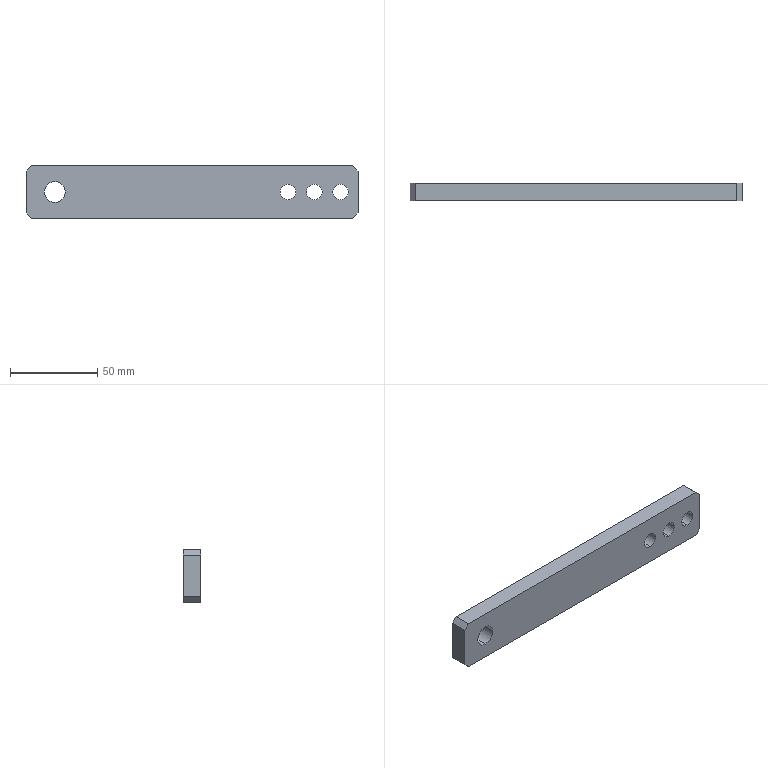Part | SolidWorks | features HoleWzd 2, Chamfer 1, Extrusion 1 | 1 solid | 18 faces | box 190 x 10 x 30 mm | volume 53781 mm3 | plane 10 | cylinder 8 | commonest cylinder face diameters 9 x6 12 x2
STEP:
#1=CARTESIAN_POINT('',(-78.492,10.,-6.));
#2=VERTEX_POINT('',#1);
#3=CARTESIAN_POINT('',(-78.492,10.,6.));
#4=VERTEX_POINT('',#3);
#5=CARTESIAN_POINT('',(-78.492,10.,0.));
#6=DIRECTION('',(0.,1.,0.));
#7=DIRECTION('',(0.,0.,1.));
#8=AXIS2_PLACEMENT_3D('',#5,#6,#7);
#9=CIRCLE('',#8,6.);
#10=EDGE_CURVE('',#2,#4,#9,.T.);
#11=ORIENTED_EDGE('',*,*,#10,.T.);
#12=CARTESIAN_POINT('',(-78.492,0.,6.));
#13=VERTEX_POINT('',#12);
#14=CARTESIAN_POINT('',(-78.492,0.,6.));
#15=DIRECTION('',(0.,-1.,0.));
#16=VECTOR('',#15,1000.);
#17=LINE('',#14,#16);
#18=EDGE_CURVE('',#4,#13,#17,.T.);
#19=ORIENTED_EDGE('',*,*,#18,.T.);
#20=CARTESIAN_POINT('',(-78.492,0.,-6.));
#21=VERTEX_POINT('',#20);
#22=CARTESIAN_POINT('',(-78.492,0.,0.));
#23=DIRECTION('',(0.,-1.,0.));
#24=DIRECTION('',(0.,0.,-1.));
#25=AXIS2_PLACEMENT_3D('',#22,#23,#24);
#26=CIRCLE('',#25,6.);
#27=EDGE_CURVE('',#13,#21,#26,.T.);
#28=ORIENTED_EDGE('',*,*,#27,.T.);
#29=CARTESIAN_POINT('',(-78.492,0.,-6.));
#30=DIRECTION('',(0.,-1.,0.));
#31=VECTOR('',#30,1000.);
#32=LINE('',#29,#31);
#33=EDGE_CURVE('',#2,#21,#32,.T.);
#34=ORIENTED_EDGE('',*,*,#33,.F.);
#35=EDGE_LOOP('',(#11,#19,#28,#34));
#36=FACE_OUTER_BOUND('',#35,.T.);
#37=CARTESIAN_POINT('',(-78.492,0.,0.));
#38=DIRECTION('',(0.,-1.,0.));
#39=DIRECTION('',(0.,0.,-1.));
#40=AXIS2_PLACEMENT_3D('',#37,#38,#39);
#41=CYLINDRICAL_SURFACE('',#40,6.);
#42=ADVANCED_FACE('',(#36),#41,.F.);
#43=CARTESIAN_POINT('',(85.,0.,-4.5));
#44=VERTEX_POINT('',#43);
#45=CARTESIAN_POINT('',(85.,0.,4.5));
#46=VERTEX_POINT('',#45);
#47=CARTESIAN_POINT('',(85.,0.,0.));
#48=DIRECTION('',(0.,1.,0.));
#49=DIRECTION('',(0.,0.,1.));
#50=AXIS2_PLACEMENT_3D('',#47,#48,#49);
#51=CIRCLE('',#50,4.5);
#52=EDGE_CURVE('',#44,#46,#51,.T.);
#53=ORIENTED_EDGE('',*,*,#52,.F.);
#54=CARTESIAN_POINT('',(85.,10.,-4.5));
#55=VERTEX_POINT('',#54);
#56=CARTESIAN_POINT('',(85.,10.,-4.5));
#57=DIRECTION('',(0.,1.,0.));
#58=VECTOR('',#57,1000.);
#59=LINE('',#56,#58);
#60=EDGE_CURVE('',#44,#55,#59,.T.);
#61=ORIENTED_EDGE('',*,*,#60,.T.);
#62=CARTESIAN_POINT('',(85.,10.,4.5));
#63=VERTEX_POINT('',#62);
#64=CARTESIAN_POINT('',(85.,10.,0.));
#65=DIRECTION('',(0.,1.,0.));
#66=DIRECTION('',(0.,0.,1.));
#67=AXIS2_PLACEMENT_3D('',#64,#65,#66);
#68=CIRCLE('',#67,4.5);
#69=EDGE_CURVE('',#55,#63,#68,.T.);
#70=ORIENTED_EDGE('',*,*,#69,.T.);
#71=CARTESIAN_POINT('',(85.,10.,4.5));
#72=DIRECTION('',(0.,1.,0.));
#73=VECTOR('',#72,1000.);
#74=LINE('',#71,#73);
#75=EDGE_CURVE('',#46,#63,#74,.T.);
#76=ORIENTED_EDGE('',*,*,#75,.F.);
#77=EDGE_LOOP('',(#53,#61,#70,#76));
#78=FACE_OUTER_BOUND('',#77,.T.);
#79=CARTESIAN_POINT('',(85.,10.,0.));
#80=DIRECTION('',(0.,1.,0.));
#81=DIRECTION('',(0.,0.,1.));
#82=AXIS2_PLACEMENT_3D('',#79,#80,#81);
#83=CYLINDRICAL_SURFACE('',#82,4.5);
#84=ADVANCED_FACE('',(#78),#83,.F.);
#85=CARTESIAN_POINT('',(70.,0.,-4.5));
#86=VERTEX_POINT('',#85);
#87=CARTESIAN_POINT('',(70.,0.,4.5));
#88=VERTEX_POINT('',#87);
#89=CARTESIAN_POINT('',(70.,0.,0.));
#90=DIRECTION('',(0.,1.,0.));
#91=DIRECTION('',(0.,0.,1.));
#92=AXIS2_PLACEMENT_3D('',#89,#90,#91);
#93=CIRCLE('',#92,4.5);
#94=EDGE_CURVE('',#86,#88,#93,.T.);
#95=ORIENTED_EDGE('',*,*,#94,.F.);
#96=CARTESIAN_POINT('',(70.,10.,-4.5));
#97=VERTEX_POINT('',#96);
#98=CARTESIAN_POINT('',(70.,10.,-4.5));
#99=DIRECTION('',(0.,1.,0.));
#100=VECTOR('',#99,1000.);
#101=LINE('',#98,#100);
#102=EDGE_CURVE('',#86,#97,#101,.T.);
#103=ORIENTED_EDGE('',*,*,#102,.T.);
#104=CARTESIAN_POINT('',(70.,10.,4.5));
#105=VERTEX_POINT('',#104);
#106=CARTESIAN_POINT('',(70.,10.,0.));
#107=DIRECTION('',(0.,1.,0.));
#108=DIRECTION('',(0.,0.,1.));
#109=AXIS2_PLACEMENT_3D('',#106,#107,#108);
#110=CIRCLE('',#109,4.5);
#111=EDGE_CURVE('',#97,#105,#110,.T.);
#112=ORIENTED_EDGE('',*,*,#111,.T.);
#113=CARTESIAN_POINT('',(70.,10.,4.5));
#114=DIRECTION('',(0.,1.,0.));
#115=VECTOR('',#114,1000.);
#116=LINE('',#113,#115);
#117=EDGE_CURVE('',#88,#105,#116,.T.);
#118=ORIENTED_EDGE('',*,*,#117,.F.);
#119=EDGE_LOOP('',(#95,#103,#112,#118));
#120=FACE_OUTER_BOUND('',#119,.T.);
#121=CARTESIAN_POINT('',(70.,10.,0.));
#122=DIRECTION('',(0.,1.,0.));
#123=DIRECTION('',(0.,0.,1.));
#124=AXIS2_PLACEMENT_3D('',#121,#122,#123);
#125=CYLINDRICAL_SURFACE('',#124,4.5);
#126=ADVANCED_FACE('',(#120),#125,.F.);
#127=CARTESIAN_POINT('',(55.,0.,-4.5));
#128=VERTEX_POINT('',#127);
#129=CARTESIAN_POINT('',(55.,0.,4.5));
#130=VERTEX_POINT('',#129);
#131=CARTESIAN_POINT('',(55.,0.,0.));
#132=DIRECTION('',(0.,1.,0.));
#133=DIRECTION('',(0.,0.,1.));
#134=AXIS2_PLACEMENT_3D('',#131,#132,#133);
#135=CIRCLE('',#134,4.5);
#136=EDGE_CURVE('',#128,#130,#135,.T.);
#137=ORIENTED_EDGE('',*,*,#136,.F.);
#138=CARTESIAN_POINT('',(55.,10.,-4.5));
#139=VERTEX_POINT('',#138);
#140=CARTESIAN_POINT('',(55.,10.,-4.5));
#141=DIRECTION('',(0.,1.,0.));
#142=VECTOR('',#141,1000.);
#143=LINE('',#140,#142);
#144=EDGE_CURVE('',#128,#139,#143,.T.);
#145=ORIENTED_EDGE('',*,*,#144,.T.);
#146=CARTESIAN_POINT('',(55.,10.,4.5));
#147=VERTEX_POINT('',#146);
#148=CARTESIAN_POINT('',(55.,10.,0.));
#149=DIRECTION('',(0.,1.,0.));
#150=DIRECTION('',(0.,0.,1.));
#151=AXIS2_PLACEMENT_3D('',#148,#149,#150);
#152=CIRCLE('',#151,4.5);
#153=EDGE_CURVE('',#139,#147,#152,.T.);
#154=ORIENTED_EDGE('',*,*,#153,.T.);
#155=CARTESIAN_POINT('',(55.,10.,4.5));
#156=DIRECTION('',(0.,1.,0.));
#157=VECTOR('',#156,1000.);
#158=LINE('',#155,#157);
#159=EDGE_CURVE('',#130,#147,#158,.T.);
#160=ORIENTED_EDGE('',*,*,#159,.F.);
#161=EDGE_LOOP('',(#137,#145,#154,#160));
#162=FACE_OUTER_BOUND('',#161,.T.);
#163=CARTESIAN_POINT('',(55.,10.,0.));
#164=DIRECTION('',(0.,1.,0.));
#165=DIRECTION('',(0.,0.,1.));
#166=AXIS2_PLACEMENT_3D('',#163,#164,#165);
#167=CYLINDRICAL_SURFACE('',#166,4.5);
#168=ADVANCED_FACE('',(#162),#167,.F.);
#169=CARTESIAN_POINT('',(95.,0.,12.));
#170=VERTEX_POINT('',#169);
#171=CARTESIAN_POINT('',(95.,0.,-12.));
#172=VERTEX_POINT('',#171);
#173=CARTESIAN_POINT('',(95.,0.,-15.));
#174=DIRECTION('',(0.,0.,-1.));
#175=VECTOR('',#174,1000.);
#176=LINE('',#173,#175);
#177=EDGE_CURVE('',#170,#172,#176,.T.);
#178=ORIENTED_EDGE('',*,*,#177,.T.);
#179=CARTESIAN_POINT('',(95.,10.,-12.));
#180=VERTEX_POINT('',#179);
#181=CARTESIAN_POINT('',(95.,10.,-12.));
#182=DIRECTION('',(0.,1.,0.));
#183=VECTOR('',#182,1000.);
#184=LINE('',#181,#183);
#185=EDGE_CURVE('',#172,#180,#184,.T.);
#186=ORIENTED_EDGE('',*,*,#185,.T.);
#187=CARTESIAN_POINT('',(95.,10.,12.));
#188=VERTEX_POINT('',#187);
#189=CARTESIAN_POINT('',(95.,10.,-15.));
#190=DIRECTION('',(0.,0.,-1.));
#191=VECTOR('',#190,1000.);
#192=LINE('',#189,#191);
#193=EDGE_CURVE('',#188,#180,#192,.T.);
#194=ORIENTED_EDGE('',*,*,#193,.F.);
#195=CARTESIAN_POINT('',(95.,10.,12.));
#196=DIRECTION('',(0.,-1.,0.));
#197=VECTOR('',#196,1000.);
#198=LINE('',#195,#197);
#199=EDGE_CURVE('',#188,#170,#198,.T.);
#200=ORIENTED_EDGE('',*,*,#199,.T.);
#201=EDGE_LOOP('',(#178,#186,#194,#200));
#202=FACE_OUTER_BOUND('',#201,.T.);
#203=CARTESIAN_POINT('',(95.,10.,-15.));
#204=DIRECTION('',(-1.,0.,0.));
#205=DIRECTION('',(0.,0.,1.));
#206=AXIS2_PLACEMENT_3D('',#203,#204,#205);
#207=PLANE('',#206);
#208=ADVANCED_FACE('',(#202),#207,.F.);
#209=CARTESIAN_POINT('',(92.,0.,-15.));
#210=VERTEX_POINT('',#209);
#211=CARTESIAN_POINT('',(-92.,0.,-15.));
#212=VERTEX_POINT('',#211);
#213=CARTESIAN_POINT('',(-95.,0.,-15.));
#214=DIRECTION('',(-1.,0.,0.));
#215=VECTOR('',#214,1000.);
#216=LINE('',#213,#215);
#217=EDGE_CURVE('',#210,#212,#216,.T.);
#218=ORIENTED_EDGE('',*,*,#217,.T.);
#219=CARTESIAN_POINT('',(-92.,10.,-15.));
#220=VERTEX_POINT('',#219);
#221=CARTESIAN_POINT('',(-92.,10.,-15.));
#222=DIRECTION('',(0.,1.,0.));
#223=VECTOR('',#222,1000.);
#224=LINE('',#221,#223);
#225=EDGE_CURVE('',#212,#220,#224,.T.);
#226=ORIENTED_EDGE('',*,*,#225,.T.);
#227=CARTESIAN_POINT('',(92.,10.,-15.));
#228=VERTEX_POINT('',#227);
#229=CARTESIAN_POINT('',(-95.,10.,-15.));
#230=DIRECTION('',(-1.,0.,0.));
#231=VECTOR('',#230,1000.);
#232=LINE('',#229,#231);
#233=EDGE_CURVE('',#228,#220,#232,.T.);
#234=ORIENTED_EDGE('',*,*,#233,.F.);
#235=CARTESIAN_POINT('',(92.,10.,-15.));
#236=DIRECTION('',(0.,-1.,0.));
#237=VECTOR('',#236,1000.);
#238=LINE('',#235,#237);
#239=EDGE_CURVE('',#228,#210,#238,.T.);
#240=ORIENTED_EDGE('',*,*,#239,.T.);
#241=EDGE_LOOP('',(#218,#226,#234,#240));
#242=FACE_OUTER_BOUND('',#241,.T.);
#243=CARTESIAN_POINT('',(-95.,10.,-15.));
#244=DIRECTION('',(0.,0.,1.));
#245=DIRECTION('',(1.,0.,0.));
#246=AXIS2_PLACEMENT_3D('',#243,#244,#245);
#247=PLANE('',#246);
#248=ADVANCED_FACE('',(#242),#247,.F.);
#249=CARTESIAN_POINT('',(-95.,10.,-12.));
#250=VERTEX_POINT('',#249);
#251=CARTESIAN_POINT('',(-95.,10.,12.));
#252=VERTEX_POINT('',#251);
#253=CARTESIAN_POINT('',(-95.,10.,-15.));
#254=DIRECTION('',(0.,0.,1.));
#255=VECTOR('',#254,1000.);
#256=LINE('',#253,#255);
#257=EDGE_CURVE('',#250,#252,#256,.T.);
#258=ORIENTED_EDGE('',*,*,#257,.F.);
#259=CARTESIAN_POINT('',(-95.,0.,-12.));
#260=VERTEX_POINT('',#259);
#261=CARTESIAN_POINT('',(-95.,10.,-12.));
#262=DIRECTION('',(0.,-1.,0.));
#263=VECTOR('',#262,1000.);
#264=LINE('',#261,#263);
#265=EDGE_CURVE('',#250,#260,#264,.T.);
#266=ORIENTED_EDGE('',*,*,#265,.T.);
#267=CARTESIAN_POINT('',(-95.,0.,12.));
#268=VERTEX_POINT('',#267);
#269=CARTESIAN_POINT('',(-95.,0.,-15.));
#270=DIRECTION('',(0.,0.,1.));
#271=VECTOR('',#270,1000.);
#272=LINE('',#269,#271);
#273=EDGE_CURVE('',#260,#268,#272,.T.);
#274=ORIENTED_EDGE('',*,*,#273,.T.);
#275=CARTESIAN_POINT('',(-95.,10.,12.));
#276=DIRECTION('',(0.,1.,0.));
#277=VECTOR('',#276,1000.);
#278=LINE('',#275,#277);
#279=EDGE_CURVE('',#268,#252,#278,.T.);
#280=ORIENTED_EDGE('',*,*,#279,.T.);
#281=EDGE_LOOP('',(#258,#266,#274,#280));
#282=FACE_OUTER_BOUND('',#281,.T.);
#283=CARTESIAN_POINT('',(-95.,10.,-15.));
#284=DIRECTION('',(1.,0.,0.));
#285=DIRECTION('',(0.,0.,-1.));
#286=AXIS2_PLACEMENT_3D('',#283,#284,#285);
#287=PLANE('',#286);
#288=ADVANCED_FACE('',(#282),#287,.F.);
#289=CARTESIAN_POINT('',(-92.,0.,15.));
#290=VERTEX_POINT('',#289);
#291=CARTESIAN_POINT('',(92.,0.,15.));
#292=VERTEX_POINT('',#291);
#293=CARTESIAN_POINT('',(-95.,0.,15.));
#294=DIRECTION('',(1.,0.,0.));
#295=VECTOR('',#294,1000.);
#296=LINE('',#293,#295);
#297=EDGE_CURVE('',#290,#292,#296,.T.);
#298=ORIENTED_EDGE('',*,*,#297,.T.);
#299=CARTESIAN_POINT('',(92.,10.,15.));
#300=VERTEX_POINT('',#299);
#301=CARTESIAN_POINT('',(92.,10.,15.));
#302=DIRECTION('',(0.,1.,0.));
#303=VECTOR('',#302,1000.);
#304=LINE('',#301,#303);
#305=EDGE_CURVE('',#292,#300,#304,.T.);
#306=ORIENTED_EDGE('',*,*,#305,.T.);
#307=CARTESIAN_POINT('',(-92.,10.,15.));
#308=VERTEX_POINT('',#307);
#309=CARTESIAN_POINT('',(-95.,10.,15.));
#310=DIRECTION('',(1.,0.,0.));
#311=VECTOR('',#310,1000.);
#312=LINE('',#309,#311);
#313=EDGE_CURVE('',#308,#300,#312,.T.);
#314=ORIENTED_EDGE('',*,*,#313,.F.);
#315=CARTESIAN_POINT('',(-92.,10.,15.));
#316=DIRECTION('',(0.,-1.,0.));
#317=VECTOR('',#316,1000.);
#318=LINE('',#315,#317);
#319=EDGE_CURVE('',#308,#290,#318,.T.);
#320=ORIENTED_EDGE('',*,*,#319,.T.);
#321=EDGE_LOOP('',(#298,#306,#314,#320));
#322=FACE_OUTER_BOUND('',#321,.T.);
#323=CARTESIAN_POINT('',(-95.,10.,15.));
#324=DIRECTION('',(0.,0.,-1.));
#325=DIRECTION('',(-1.,0.,0.));
#326=AXIS2_PLACEMENT_3D('',#323,#324,#325);
#327=PLANE('',#326);
#328=ADVANCED_FACE('',(#322),#327,.F.);
#329=ORIENTED_EDGE('',*,*,#10,.F.);
#330=CARTESIAN_POINT('',(-78.492,10.,0.));
#331=DIRECTION('',(0.,1.,0.));
#332=DIRECTION('',(0.,0.,1.));
#333=AXIS2_PLACEMENT_3D('',#330,#331,#332);
#334=CIRCLE('',#333,6.);
#335=EDGE_CURVE('',#4,#2,#334,.T.);
#336=ORIENTED_EDGE('',*,*,#335,.F.);
#337=EDGE_LOOP('',(#329,#336));
#338=FACE_BOUND('',#337,.T.);
#339=CARTESIAN_POINT('',(85.,10.,0.));
#340=DIRECTION('',(0.,1.,0.));
#341=DIRECTION('',(0.,0.,1.));
#342=AXIS2_PLACEMENT_3D('',#339,#340,#341);
#343=CIRCLE('',#342,4.5);
#344=EDGE_CURVE('',#63,#55,#343,.T.);
#345=ORIENTED_EDGE('',*,*,#344,.F.);
#346=ORIENTED_EDGE('',*,*,#69,.F.);
#347=EDGE_LOOP('',(#345,#346));
#348=FACE_BOUND('',#347,.T.);
#349=CARTESIAN_POINT('',(70.,10.,0.));
#350=DIRECTION('',(0.,1.,0.));
#351=DIRECTION('',(0.,0.,1.));
#352=AXIS2_PLACEMENT_3D('',#349,#350,#351);
#353=CIRCLE('',#352,4.5);
#354=EDGE_CURVE('',#105,#97,#353,.T.);
#355=ORIENTED_EDGE('',*,*,#354,.F.);
#356=ORIENTED_EDGE('',*,*,#111,.F.);
#357=EDGE_LOOP('',(#355,#356));
#358=FACE_BOUND('',#357,.T.);
#359=CARTESIAN_POINT('',(55.,10.,0.));
#360=DIRECTION('',(0.,1.,0.));
#361=DIRECTION('',(0.,0.,1.));
#362=AXIS2_PLACEMENT_3D('',#359,#360,#361);
#363=CIRCLE('',#362,4.5);
#364=EDGE_CURVE('',#147,#139,#363,.T.);
#365=ORIENTED_EDGE('',*,*,#364,.F.);
#366=ORIENTED_EDGE('',*,*,#153,.F.);
#367=EDGE_LOOP('',(#365,#366));
#368=FACE_BOUND('',#367,.T.);
#369=ORIENTED_EDGE('',*,*,#233,.T.);
#370=CARTESIAN_POINT('',(-53.5,10.,-53.5));
#371=DIRECTION('',(-0.7071,0.,0.7071));
#372=VECTOR('',#371,1000.);
#373=LINE('',#370,#372);
#374=EDGE_CURVE('',#220,#250,#373,.T.);
#375=ORIENTED_EDGE('',*,*,#374,.T.);
#376=ORIENTED_EDGE('',*,*,#257,.T.);
#377=CARTESIAN_POINT('',(-53.5,10.,53.5));
#378=DIRECTION('',(0.7071,0.,0.7071));
#379=VECTOR('',#378,1000.);
#380=LINE('',#377,#379);
#381=EDGE_CURVE('',#252,#308,#380,.T.);
#382=ORIENTED_EDGE('',*,*,#381,.T.);
#383=ORIENTED_EDGE('',*,*,#313,.T.);
#384=CARTESIAN_POINT('',(53.5,10.,53.5));
#385=DIRECTION('',(0.7071,0.,-0.7071));
#386=VECTOR('',#385,1000.);
#387=LINE('',#384,#386);
#388=EDGE_CURVE('',#300,#188,#387,.T.);
#389=ORIENTED_EDGE('',*,*,#388,.T.);
#390=ORIENTED_EDGE('',*,*,#193,.T.);
#391=CARTESIAN_POINT('',(53.5,10.,-53.5));
#392=DIRECTION('',(-0.7071,0.,-0.7071));
#393=VECTOR('',#392,1000.);
#394=LINE('',#391,#393);
#395=EDGE_CURVE('',#180,#228,#394,.T.);
#396=ORIENTED_EDGE('',*,*,#395,.T.);
#397=EDGE_LOOP('',(#369,#375,#376,#382,#383,#389,#390,#396));
#398=FACE_OUTER_BOUND('',#397,.T.);
#399=CARTESIAN_POINT('',(0.,10.,0.));
#400=DIRECTION('',(0.,1.,0.));
#401=DIRECTION('',(0.,0.,1.));
#402=AXIS2_PLACEMENT_3D('',#399,#400,#401);
#403=PLANE('',#402);
#404=ADVANCED_FACE('',(#338,#348,#358,#368,#398),#403,.T.);
#405=CARTESIAN_POINT('',(-78.492,0.,0.));
#406=DIRECTION('',(0.,-1.,0.));
#407=DIRECTION('',(0.,0.,-1.));
#408=AXIS2_PLACEMENT_3D('',#405,#406,#407);
#409=CIRCLE('',#408,6.);
#410=EDGE_CURVE('',#21,#13,#409,.T.);
#411=ORIENTED_EDGE('',*,*,#410,.F.);
#412=ORIENTED_EDGE('',*,*,#27,.F.);
#413=EDGE_LOOP('',(#411,#412));
#414=FACE_BOUND('',#413,.T.);
#415=CARTESIAN_POINT('',(85.,0.,0.));
#416=DIRECTION('',(0.,1.,0.));
#417=DIRECTION('',(0.,0.,1.));
#418=AXIS2_PLACEMENT_3D('',#415,#416,#417);
#419=CIRCLE('',#418,4.5);
#420=EDGE_CURVE('',#46,#44,#419,.T.);
#421=ORIENTED_EDGE('',*,*,#420,.T.);
#422=ORIENTED_EDGE('',*,*,#52,.T.);
#423=EDGE_LOOP('',(#421,#422));
#424=FACE_BOUND('',#423,.T.);
#425=CARTESIAN_POINT('',(70.,0.,0.));
#426=DIRECTION('',(0.,1.,0.));
#427=DIRECTION('',(0.,0.,1.));
#428=AXIS2_PLACEMENT_3D('',#425,#426,#427);
#429=CIRCLE('',#428,4.5);
#430=EDGE_CURVE('',#88,#86,#429,.T.);
#431=ORIENTED_EDGE('',*,*,#430,.T.);
#432=ORIENTED_EDGE('',*,*,#94,.T.);
#433=EDGE_LOOP('',(#431,#432));
#434=FACE_BOUND('',#433,.T.);
#435=CARTESIAN_POINT('',(55.,0.,0.));
#436=DIRECTION('',(0.,1.,0.));
#437=DIRECTION('',(0.,0.,1.));
#438=AXIS2_PLACEMENT_3D('',#435,#436,#437);
#439=CIRCLE('',#438,4.5);
#440=EDGE_CURVE('',#130,#128,#439,.T.);
#441=ORIENTED_EDGE('',*,*,#440,.T.);
#442=ORIENTED_EDGE('',*,*,#136,.T.);
#443=EDGE_LOOP('',(#441,#442));
#444=FACE_BOUND('',#443,.T.);
#445=ORIENTED_EDGE('',*,*,#273,.F.);
#446=CARTESIAN_POINT('',(-95.,0.,-12.));
#447=DIRECTION('',(0.7071,0.,-0.7071));
#448=VECTOR('',#447,1000.);
#449=LINE('',#446,#448);
#450=EDGE_CURVE('',#260,#212,#449,.T.);
#451=ORIENTED_EDGE('',*,*,#450,.T.);
#452=ORIENTED_EDGE('',*,*,#217,.F.);
#453=CARTESIAN_POINT('',(92.,0.,-15.));
#454=DIRECTION('',(0.7071,0.,0.7071));
#455=VECTOR('',#454,1000.);
#456=LINE('',#453,#455);
#457=EDGE_CURVE('',#210,#172,#456,.T.);
#458=ORIENTED_EDGE('',*,*,#457,.T.);
#459=ORIENTED_EDGE('',*,*,#177,.F.);
#460=CARTESIAN_POINT('',(95.,0.,12.));
#461=DIRECTION('',(-0.7071,0.,0.7071));
#462=VECTOR('',#461,1000.);
#463=LINE('',#460,#462);
#464=EDGE_CURVE('',#170,#292,#463,.T.);
#465=ORIENTED_EDGE('',*,*,#464,.T.);
#466=ORIENTED_EDGE('',*,*,#297,.F.);
#467=CARTESIAN_POINT('',(-92.,0.,15.));
#468=DIRECTION('',(-0.7071,0.,-0.7071));
#469=VECTOR('',#468,1000.);
#470=LINE('',#467,#469);
#471=EDGE_CURVE('',#290,#268,#470,.T.);
#472=ORIENTED_EDGE('',*,*,#471,.T.);
#473=EDGE_LOOP('',(#445,#451,#452,#458,#459,#465,#466,#472));
#474=FACE_OUTER_BOUND('',#473,.T.);
#475=CARTESIAN_POINT('',(0.,0.,0.));
#476=DIRECTION('',(0.,1.,0.));
#477=DIRECTION('',(0.,0.,1.));
#478=AXIS2_PLACEMENT_3D('',#475,#476,#477);
#479=PLANE('',#478);
#480=ADVANCED_FACE('',(#414,#424,#434,#444,#474),#479,.F.);
#481=ORIENTED_EDGE('',*,*,#374,.F.);
#482=ORIENTED_EDGE('',*,*,#225,.F.);
#483=ORIENTED_EDGE('',*,*,#450,.F.);
#484=ORIENTED_EDGE('',*,*,#265,.F.);
#485=EDGE_LOOP('',(#481,#482,#483,#484));
#486=FACE_OUTER_BOUND('',#485,.T.);
#487=CARTESIAN_POINT('',(-95.,10.,-12.));
#488=DIRECTION('',(0.7071,0.,0.7071));
#489=DIRECTION('',(0.,-1.,0.));
#490=AXIS2_PLACEMENT_3D('',#487,#488,#489);
#491=PLANE('',#490);
#492=ADVANCED_FACE('',(#486),#491,.F.);
#493=ORIENTED_EDGE('',*,*,#395,.F.);
#494=ORIENTED_EDGE('',*,*,#185,.F.);
#495=ORIENTED_EDGE('',*,*,#457,.F.);
#496=ORIENTED_EDGE('',*,*,#239,.F.);
#497=EDGE_LOOP('',(#493,#494,#495,#496));
#498=FACE_OUTER_BOUND('',#497,.T.);
#499=CARTESIAN_POINT('',(92.,10.,-15.));
#500=DIRECTION('',(-0.7071,0.,0.7071));
#501=DIRECTION('',(0.,-1.,0.));
#502=AXIS2_PLACEMENT_3D('',#499,#500,#501);
#503=PLANE('',#502);
#504=ADVANCED_FACE('',(#498),#503,.F.);
#505=ORIENTED_EDGE('',*,*,#388,.F.);
#506=ORIENTED_EDGE('',*,*,#305,.F.);
#507=ORIENTED_EDGE('',*,*,#464,.F.);
#508=ORIENTED_EDGE('',*,*,#199,.F.);
#509=EDGE_LOOP('',(#505,#506,#507,#508));
#510=FACE_OUTER_BOUND('',#509,.T.);
#511=CARTESIAN_POINT('',(95.,10.,12.));
#512=DIRECTION('',(-0.7071,0.,-0.7071));
#513=DIRECTION('',(0.,-1.,0.));
#514=AXIS2_PLACEMENT_3D('',#511,#512,#513);
#515=PLANE('',#514);
#516=ADVANCED_FACE('',(#510),#515,.F.);
#517=ORIENTED_EDGE('',*,*,#381,.F.);
#518=ORIENTED_EDGE('',*,*,#279,.F.);
#519=ORIENTED_EDGE('',*,*,#471,.F.);
#520=ORIENTED_EDGE('',*,*,#319,.F.);
#521=EDGE_LOOP('',(#517,#518,#519,#520));
#522=FACE_OUTER_BOUND('',#521,.T.);
#523=CARTESIAN_POINT('',(-92.,10.,15.));
#524=DIRECTION('',(0.7071,0.,-0.7071));
#525=DIRECTION('',(0.,-1.,0.));
#526=AXIS2_PLACEMENT_3D('',#523,#524,#525);
#527=PLANE('',#526);
#528=ADVANCED_FACE('',(#522),#527,.F.);
#529=ORIENTED_EDGE('',*,*,#144,.F.);
#530=ORIENTED_EDGE('',*,*,#440,.F.);
#531=ORIENTED_EDGE('',*,*,#159,.T.);
#532=ORIENTED_EDGE('',*,*,#364,.T.);
#533=EDGE_LOOP('',(#529,#530,#531,#532));
#534=FACE_OUTER_BOUND('',#533,.T.);
#535=CARTESIAN_POINT('',(55.,10.,0.));
#536=DIRECTION('',(0.,1.,0.));
#537=DIRECTION('',(0.,0.,1.));
#538=AXIS2_PLACEMENT_3D('',#535,#536,#537);
#539=CYLINDRICAL_SURFACE('',#538,4.5);
#540=ADVANCED_FACE('',(#534),#539,.F.);
#541=ORIENTED_EDGE('',*,*,#102,.F.);
#542=ORIENTED_EDGE('',*,*,#430,.F.);
#543=ORIENTED_EDGE('',*,*,#117,.T.);
#544=ORIENTED_EDGE('',*,*,#354,.T.);
#545=EDGE_LOOP('',(#541,#542,#543,#544));
#546=FACE_OUTER_BOUND('',#545,.T.);
#547=CARTESIAN_POINT('',(70.,10.,0.));
#548=DIRECTION('',(0.,1.,0.));
#549=DIRECTION('',(0.,0.,1.));
#550=AXIS2_PLACEMENT_3D('',#547,#548,#549);
#551=CYLINDRICAL_SURFACE('',#550,4.5);
#552=ADVANCED_FACE('',(#546),#551,.F.);
#553=ORIENTED_EDGE('',*,*,#60,.F.);
#554=ORIENTED_EDGE('',*,*,#420,.F.);
#555=ORIENTED_EDGE('',*,*,#75,.T.);
#556=ORIENTED_EDGE('',*,*,#344,.T.);
#557=EDGE_LOOP('',(#553,#554,#555,#556));
#558=FACE_OUTER_BOUND('',#557,.T.);
#559=CARTESIAN_POINT('',(85.,10.,0.));
#560=DIRECTION('',(0.,1.,0.));
#561=DIRECTION('',(0.,0.,1.));
#562=AXIS2_PLACEMENT_3D('',#559,#560,#561);
#563=CYLINDRICAL_SURFACE('',#562,4.5);
#564=ADVANCED_FACE('',(#558),#563,.F.);
#565=ORIENTED_EDGE('',*,*,#18,.F.);
#566=ORIENTED_EDGE('',*,*,#335,.T.);
#567=ORIENTED_EDGE('',*,*,#33,.T.);
#568=ORIENTED_EDGE('',*,*,#410,.T.);
#569=EDGE_LOOP('',(#565,#566,#567,#568));
#570=FACE_OUTER_BOUND('',#569,.T.);
#571=CARTESIAN_POINT('',(-78.492,0.,0.));
#572=DIRECTION('',(0.,-1.,0.));
#573=DIRECTION('',(0.,0.,-1.));
#574=AXIS2_PLACEMENT_3D('',#571,#572,#573);
#575=CYLINDRICAL_SURFACE('',#574,6.);
#576=ADVANCED_FACE('',(#570),#575,.F.);
#577=CLOSED_SHELL('',(#42,#84,#126,#168,#208,#248,#288,#328,#404,#480,#492,#504,#516,#528,#540,#552,#564,#576));
#578=MANIFOLD_SOLID_BREP('',#577);
#579=CARTESIAN_POINT('',(0.,0.,0.));
#580=DIRECTION('',(0.,0.,1.));
#581=DIRECTION('',(1.,0.,0.));
#582=AXIS2_PLACEMENT_3D('',#579,#580,#581);
#583=(LENGTH_UNIT()NAMED_UNIT(*)SI_UNIT(.MILLI.,.METRE.));
#584=UNCERTAINTY_MEASURE_WITH_UNIT(LENGTH_MEASURE(0.00001),#583,'','');
#585=(NAMED_UNIT(*)PLANE_ANGLE_UNIT()SI_UNIT($,.RADIAN.));
#586=(NAMED_UNIT(*)SI_UNIT($,.STERADIAN.)SOLID_ANGLE_UNIT());
#587=(GEOMETRIC_REPRESENTATION_CONTEXT(3)GLOBAL_UNCERTAINTY_ASSIGNED_CONTEXT((#584))GLOBAL_UNIT_ASSIGNED_CONTEXT((#583,#585,#586))REPRESENTATION_CONTEXT('',''));
#588=ADVANCED_BREP_SHAPE_REPRESENTATION('',(#578,#582),#587);